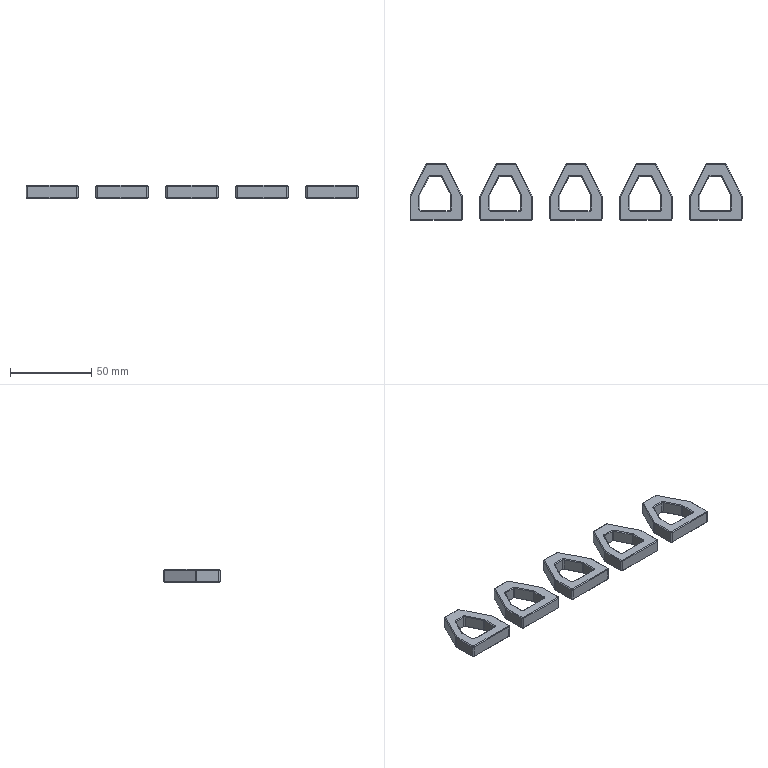NC program | NX | posted with a generic post | part box 204 x 35 x 8 mm
Lines 3514 to 3700 of 15564:
(ZLEVEL_PROFILE_COPY_1_COPY , TOOL : D10JING)
N7014 T14 M6
N7016 G54
N7018 G17 G0 G90 X43.584 Y3.5 S9500 M3
N7020 G43 Z30. H14
N7022 Z-7.
N7024 G94 G1 Z-8. F1000.
N7026 X43.664 Y4.
N7028 G3 X42.798 Y4.5 R1.
N7030 G1 X39. Y-3.097 F1200.
N7032 Y-6.5
N7034 X48.
N7036 Y-3.097
N7038 X44.202 Y4.5
N7040 X42.798
N7042 G3 X42.858 Y3.502 R1.
N7044 G1 X43.176 Y3.02
N7046 Z-7.
N7048 G0 Z53.
N7050 X89.845 Y-5.5
N7052 Z-7.
N7054 G1 Z-8. F1000.
N7056 X90.134 Y-6.
N7058 G3 X91. Y-6.5 R1.
N7060 G1 Y-3.097 F1200.
N7062 X87.202 Y4.5
N7064 X85.798
N7066 X82. Y-3.097
N7068 Y-6.5
N7070 X91.
N7072 G3 X90.5 Y-5.634 R1.
N7074 G1 X90. Y-5.345
N7076 Z-7.
N7078 G0 Z53.
N7080 X3.845 Y-5.5
N7082 Z-7.
N7084 G1 Z-8. F1000.
N7086 X4.134 Y-6.
N7088 G3 X5. Y-6.5 R1.
N7090 G1 Y-3.097 F1200.
N7092 X1.202 Y4.5
N7094 X-0.202
N7096 X-4. Y-3.097
N7098 Y-6.5
N7100 X5.
N7102 G3 X4.5 Y-5.634 R1.
N7104 G1 X4. Y-5.345
N7106 Z-7.
N7108 G0 Z53.
N7110 X-85.416 Y3.5
N7112 Z-7.
N7114 G1 Z-8. F1000.
N7116 X-85.336 Y4.
N7118 G3 X-86.202 Y4.5 R1.
N7120 G1 X-90. Y-3.097 F1200.
N7122 Y-6.5
N7124 X-81.
N7126 Y-3.097
N7128 X-84.798 Y4.5
N7130 X-86.202
N7132 G3 X-86.142 Y3.502 R1.
N7134 G1 X-85.824 Y3.02
N7136 Z-7.
N7138 G0 Z53.
N7140 X-42.416 Y3.5
N7142 Z-7.
N7144 G1 Z-8. F1000.
N7146 X-42.336 Y4.
N7148 G3 X-43.202 Y4.5 R1.
N7150 G1 X-47. Y-3.097 F1200.
N7152 Y-6.5
N7154 X-38.
N7156 Y-3.097
N7158 X-41.798 Y4.5
N7160 X-43.202
N7162 G3 X-43.142 Y3.502 R1.
N7164 G1 X-42.824 Y3.02
N7166 Z-7.
N7168 G0 Z53.
N7170 X-26.896 Y-23.412
N7172 Z-7.
N7174 G1 Z-8. F1000.
N7176 X-27.134 Y-23.
N7178 G3 X-28. Y-22.5 R1.
N7180 G1 X-58. F1200.
N7182 G2 X-64. Y-16.5 R6.
N7184 G1 Y-2.736
N7186 G2 X-63.367 Y-0.053 R6.
N7188 G1 X-53.749 Y19.183
N7190 G2 X-48.382 Y22.5 R6.
N7192 G1 X-37.618
N7194 G2 X-32.251 Y19.183 R6.
N7196 G1 X-22.633 Y-0.053
N7198 G2 X-22. Y-2.736 R6.
N7200 G1 Y-16.5
N7202 G2 X-28. Y-22.5 R6.
N7204 G3 X-28.866 Y-23. R1.
N7206 G1 X-29.155 Y-23.5
N7208 Z-7.
N7210 G0 Z30.
N7212 X-69.896 Y-23.412
N7214 Z-7.
N7216 G1 Z-8. F1000.
N7218 X-70.134 Y-23.
N7220 G3 X-71. Y-22.5 R1.
N7222 G1 X-101. F1200.
N7224 G2 X-107. Y-16.5 R6.
N7226 G1 Y-2.736
N7228 G2 X-106.367 Y-0.053 R6.
N7230 G1 X-96.749 Y19.183
N7232 G2 X-91.382 Y22.5 R6.
N7234 G1 X-80.618
N7236 G2 X-75.251 Y19.183 R6.
N7238 G1 X-65.633 Y-0.053
N7240 G2 X-65. Y-2.736 R6.
N7242 G1 Y-16.5
N7244 G2 X-71. Y-22.5 R6.
N7246 G3 X-71.866 Y-23. R1.
N7248 G1 X-72.155 Y-23.5
N7250 Z-7.
N7252 G0 Z30.
N7254 X16.104 Y-23.412
N7256 Z-7.
N7258 G1 Z-8. F1000.
N7260 X15.866 Y-23.
N7262 G3 X15. Y-22.5 R1.
N7264 G1 X-15. F1200.
N7266 G2 X-21. Y-16.5 R6.
N7268 G1 Y-2.736
N7270 G2 X-20.367 Y-0.053 R6.
N7272 G1 X-10.749 Y19.183
N7274 G2 X-5.382 Y22.5 R6.
N7276 G1 X5.382
N7278 G2 X10.749 Y19.183 R6.
N7280 G1 X20.367 Y-0.053
N7282 G2 X21. Y-2.736 R6.
N7284 G1 Y-16.5
N7286 G2 X15. Y-22.5 R6.
N7288 G3 X14.134 Y-23. R1.
N7290 G1 X13.845 Y-23.5
N7292 Z-7.
N7294 G0 Z30.
N7296 X102.104 Y-23.412
N7298 Z-7.
N7300 G1 Z-8. F1000.
N7302 X101.866 Y-23.
N7304 G3 X101. Y-22.5 R1.
N7306 G1 X71. F1200.
N7308 G2 X65. Y-16.5 R6.
N7310 G1 Y-2.736
N7312 G2 X65.633 Y-0.053 R6.
N7314 G1 X75.251 Y19.183
N7316 G2 X80.618 Y22.5 R6.
N7318 G1 X91.382
N7320 G2 X96.749 Y19.183 R6.
N7322 G1 X106.367 Y-0.053
N7324 G2 X107. Y-2.736 R6.
N7326 G1 Y-16.5
N7328 G2 X101. Y-22.5 R6.
N7330 G3 X100.134 Y-23. R1.
N7332 G1 X99.845 Y-23.5
N7334 Z-7.
N7336 G0 Z30.
N7338 X59.104 Y-23.412
N7340 Z-7.
N7342 G1 Z-8. F1000.
N7344 X58.866 Y-23.
N7346 G3 X58. Y-22.5 R1.
N7348 G1 X28. F1200.
N7350 G2 X22. Y-16.5 R6.
N7352 G1 Y-2.736
N7354 G2 X22.633 Y-0.053 R6.
N7356 G1 X32.251 Y19.183
N7358 G2 X37.618 Y22.5 R6.
N7360 G1 X48.382
N7362 G2 X53.749 Y19.183 R6.
N7364 G1 X63.367 Y-0.053
N7366 G2 X64. Y-2.736 R6.
N7368 G1 Y-16.5
N7370 G2 X58. Y-22.5 R6.
N7372 G3 X57.134 Y-23. R1.
N7374 G1 X56.845 Y-23.5
N7376 Z-7.
N7378 G0 Z30.
N7380 M5